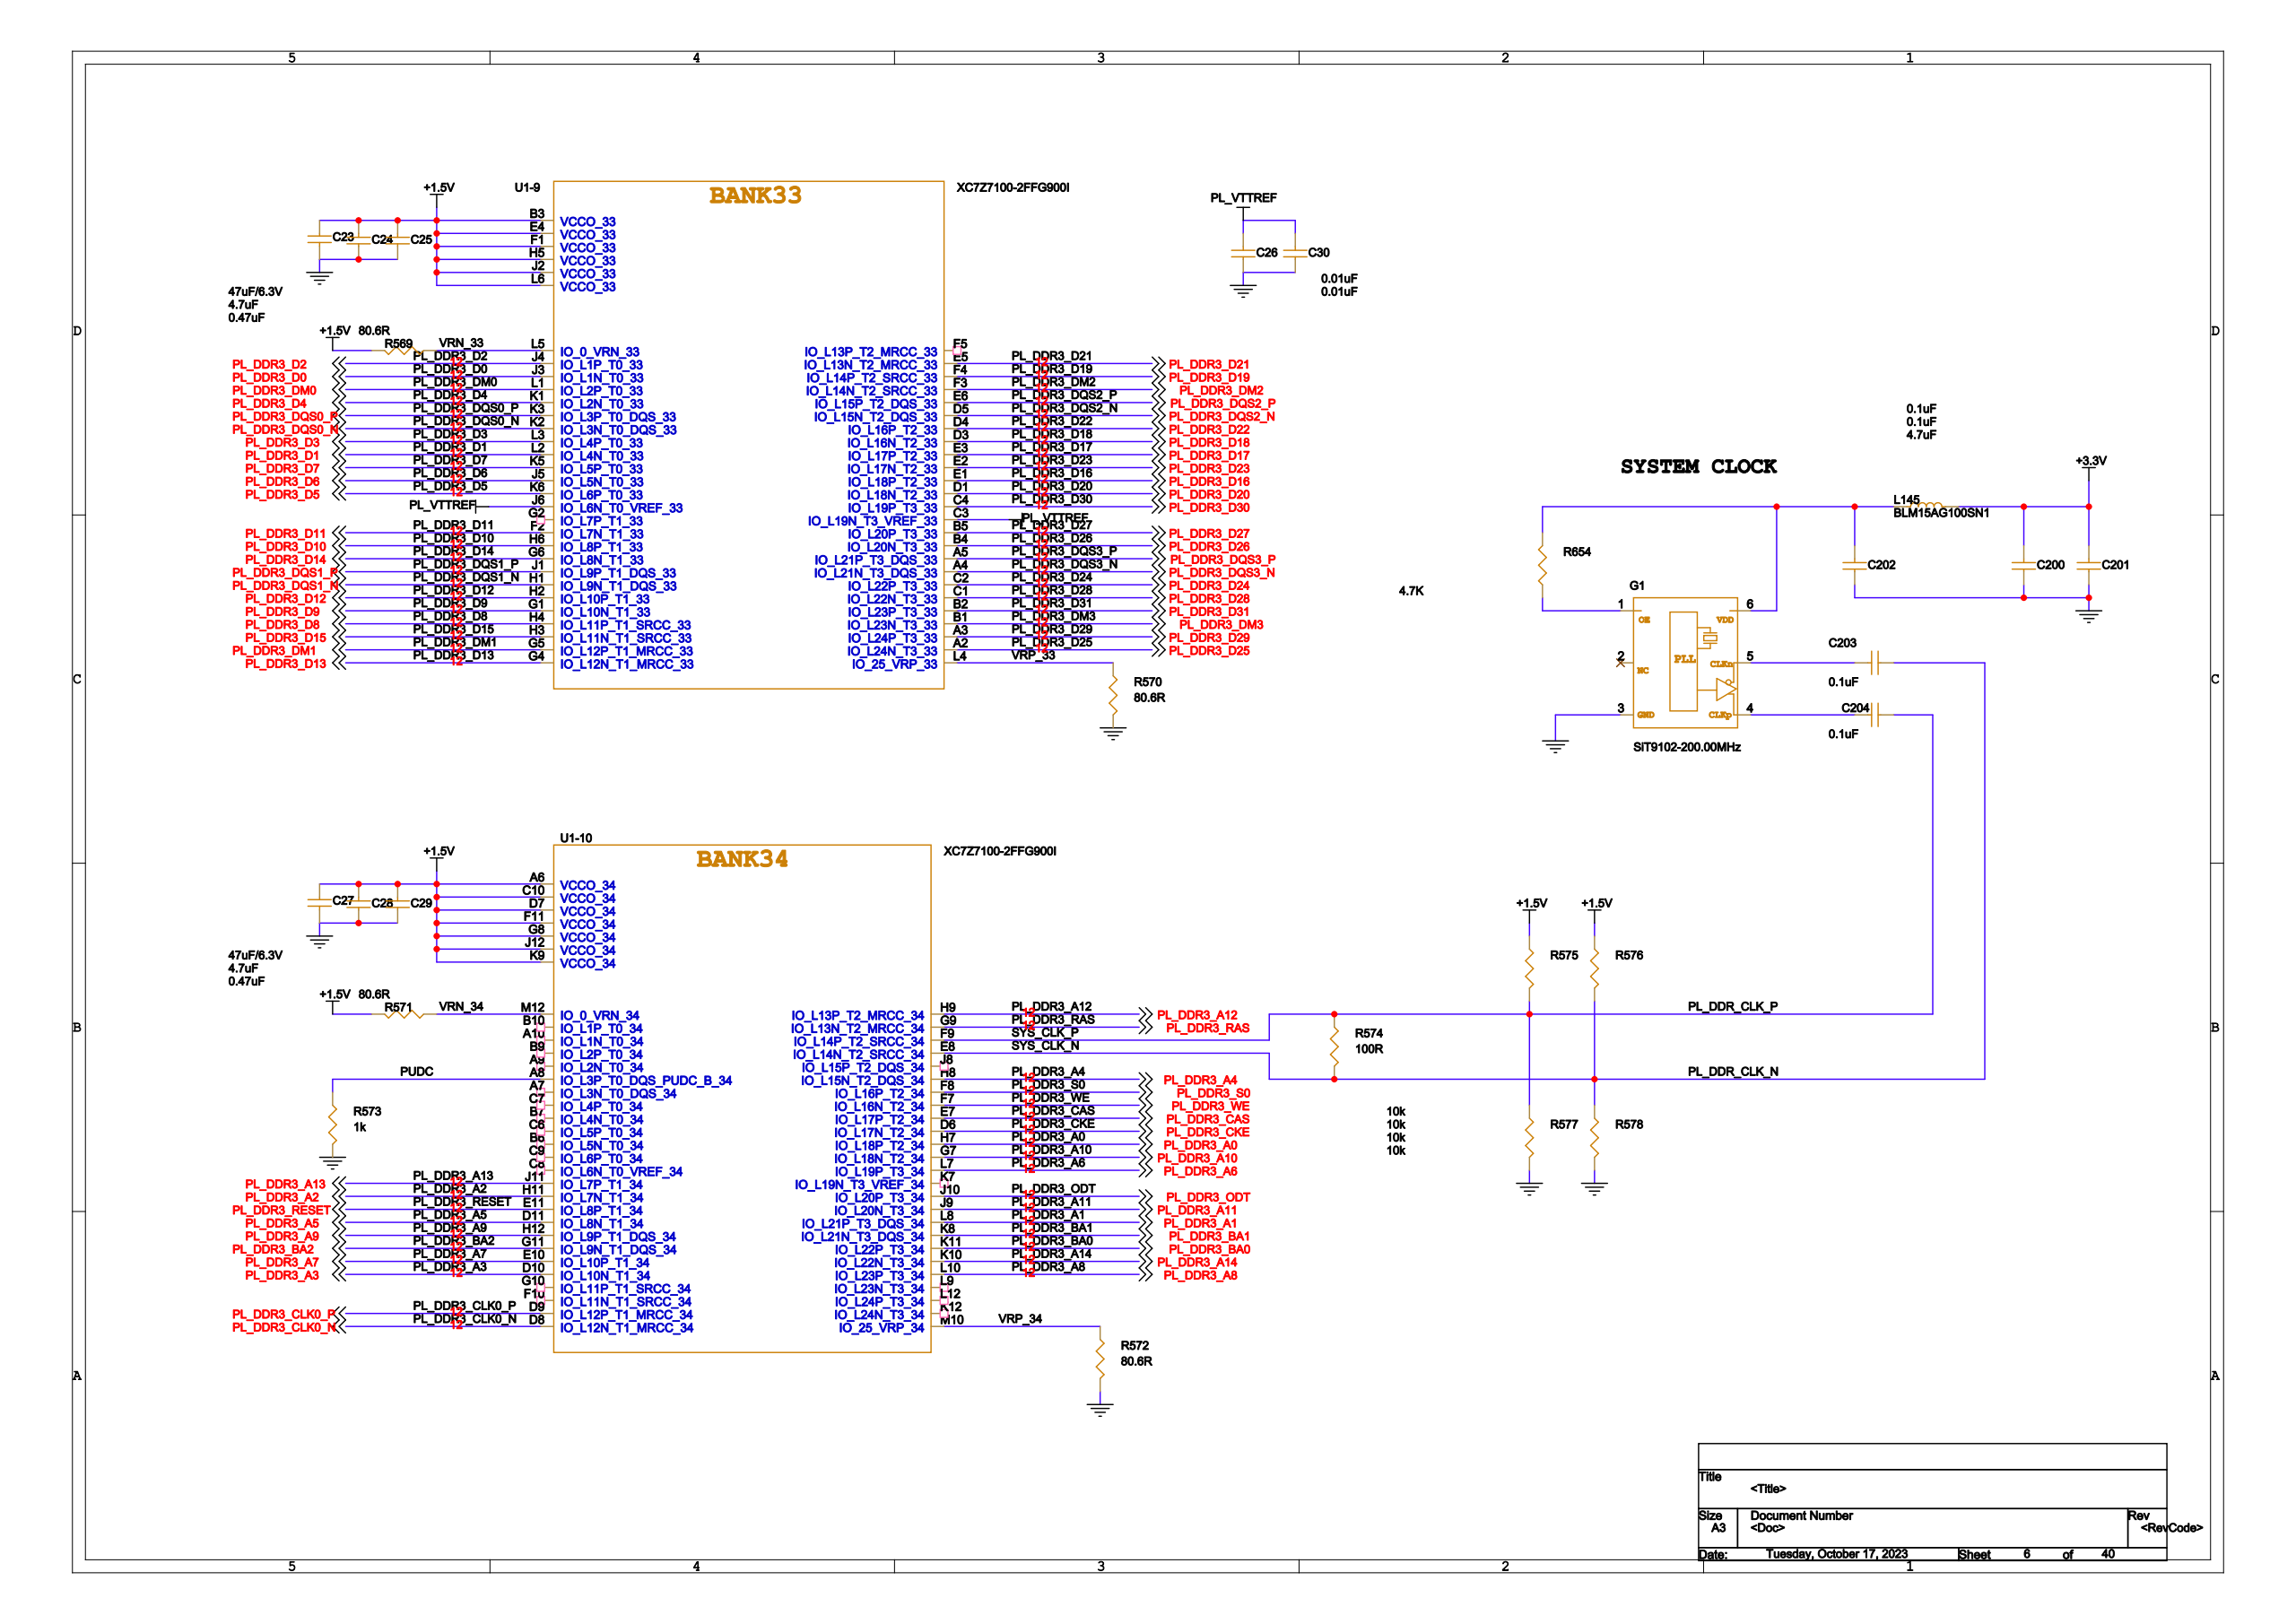Circuit board | Cadence Allegro | 1793 parts | 1223 nets | one sheet of the schematic
Parts on this sheet (reference | value | footprint):
C23 | 47uF/6.3V | C0603
C24 | 4.7uF | C0402
C25 | 0.47uF | C0402
C26 | 0.01uF | C0402
C27 | 47uF/6.3V | C0603
C28 | 4.7uF | C0402
C29 | 0.47uF | C0402
C30 | 0.01uF | C0402
C200 | 0.1uF | C0402
C201 | 4.7uF | C0402
C202 | 0.1uF | C0402
C203 | 0.1uF | C0402
C204 | 0.1uF | C0402
G1 | SiT9102-200.00MHz | OSC6-3225
L145 | BLM15AG100SN1 | L0402
R569 | 80.6R | R0402
R570 | 80.6R | R0402
R571 | 80.6R | R0402
R572 | 80.6R | R0402
R573 | 1K | R0402
R574 | 100R | R0402
R575 | 10k | R0402
R576 | 10k | R0402
R577 | 10k | R0402
R578 | 10k | R0402
R654 | 4.7K | R0402
Nets of these parts (net: part-pin ...):
GND: C23-2 C24-1 C25-1 C26-1 C27-2 C28-1 C29-1 C30-1 C200-1 C201-1 C202-1 G1-3 R570-1 R572-1 R573-1 R577-1 R578-1
+1.5V: C23-1 C24-2 C25-2 C27-1 C28-2 C29-2 R569-1 R571-1 R575-2 R576-2
+3.3V: C200-2 C201-2 L145-2
N16991426: C203-2 G1-5
N16991447: C204-2 G1-4
N16991387: G1-1 R654-2
N16991329: C202-2 G1-6 L145-1 R654-1
PL_VTTREF: C26-2 C30-2
VRN_33: R569-2
VRP_33: R570-2
VRN_34: R571-2
VRP_34: R572-2
PL_DDR_CLK_N: C203-1 R574-1 R576-1 R578-2
PL_DDR_CLK_P: C204-1 R574-2 R575-1 R577-2
PUDC: R573-2